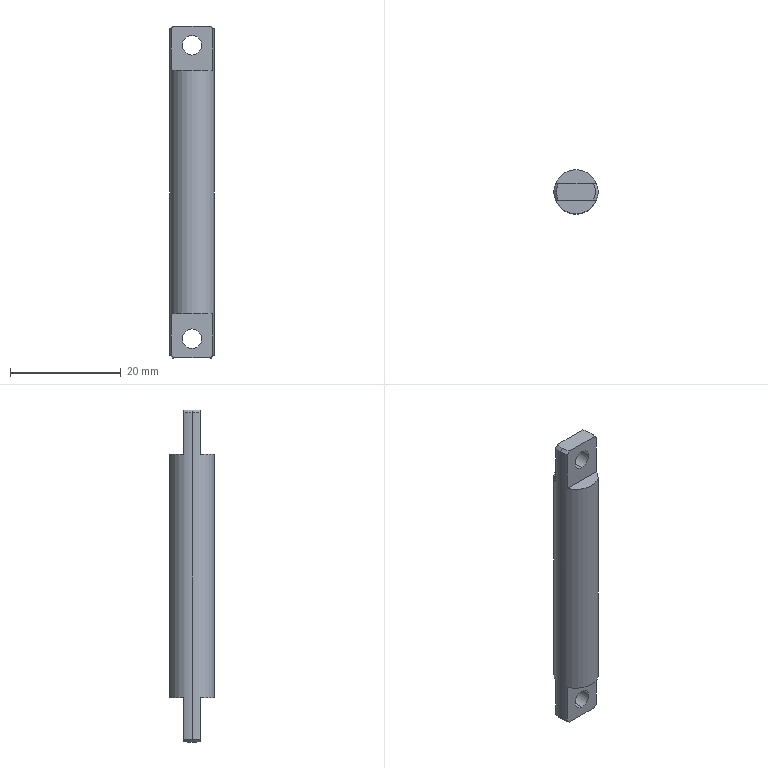Part | SolidWorks | features BaseBody 1 | 1 solid | 21 faces | box 8 x 8 x 60 mm | volume 2527 mm3 | plane 10 | cylinder 6 | cone 5 | commonest cylinder face diameters 3.5 x4 8 x2
STEP:
#1=CARTESIAN_POINT('',(4.,0.,29.5));
#2=VERTEX_POINT('',#1);
#3=CARTESIAN_POINT('',(3.708,1.5,29.5));
#4=VERTEX_POINT('',#3);
#5=CARTESIAN_POINT('',(0.,0.,29.5));
#6=DIRECTION('',(0.,0.,1.));
#7=DIRECTION('',(-1.,0.,0.));
#8=AXIS2_PLACEMENT_3D('',#5,#6,#7);
#9=CIRCLE('',#8,4.);
#10=EDGE_CURVE('',#2,#4,#9,.T.);
#11=ORIENTED_EDGE('',*,*,#10,.F.);
#12=CARTESIAN_POINT('',(4.,0.,-29.5));
#13=VERTEX_POINT('',#12);
#14=CARTESIAN_POINT('',(4.,0.,22.));
#15=DIRECTION('',(0.,0.,-1.));
#16=VECTOR('',#15,1000.);
#17=LINE('',#14,#16);
#18=EDGE_CURVE('',#2,#13,#17,.T.);
#19=ORIENTED_EDGE('',*,*,#18,.T.);
#20=CARTESIAN_POINT('',(3.708,1.5,-29.5));
#21=VERTEX_POINT('',#20);
#22=CARTESIAN_POINT('',(0.,0.,-29.5));
#23=DIRECTION('',(0.,0.,1.));
#24=DIRECTION('',(-1.,0.,0.));
#25=AXIS2_PLACEMENT_3D('',#22,#23,#24);
#26=CIRCLE('',#25,4.);
#27=EDGE_CURVE('',#13,#21,#26,.T.);
#28=ORIENTED_EDGE('',*,*,#27,.T.);
#29=CARTESIAN_POINT('',(3.708,1.5,-22.));
#30=VERTEX_POINT('',#29);
#31=CARTESIAN_POINT('',(3.708,1.5,22.));
#32=DIRECTION('',(0.,0.,1.));
#33=VECTOR('',#32,1000.);
#34=LINE('',#31,#33);
#35=EDGE_CURVE('',#21,#30,#34,.T.);
#36=ORIENTED_EDGE('',*,*,#35,.T.);
#37=CARTESIAN_POINT('',(-3.708,1.5,-22.));
#38=VERTEX_POINT('',#37);
#39=CARTESIAN_POINT('',(0.,0.,-22.));
#40=DIRECTION('',(0.,0.,1.));
#41=DIRECTION('',(-1.,0.,0.));
#42=AXIS2_PLACEMENT_3D('',#39,#40,#41);
#43=CIRCLE('',#42,4.);
#44=EDGE_CURVE('',#30,#38,#43,.T.);
#45=ORIENTED_EDGE('',*,*,#44,.T.);
#46=CARTESIAN_POINT('',(-3.708,1.5,-29.5));
#47=VERTEX_POINT('',#46);
#48=CARTESIAN_POINT('',(-3.708,1.5,22.));
#49=DIRECTION('',(0.,0.,-1.));
#50=VECTOR('',#49,1000.);
#51=LINE('',#48,#50);
#52=EDGE_CURVE('',#38,#47,#51,.T.);
#53=ORIENTED_EDGE('',*,*,#52,.T.);
#54=CARTESIAN_POINT('',(-4.,0.,-29.5));
#55=VERTEX_POINT('',#54);
#56=CARTESIAN_POINT('',(0.,0.,-29.5));
#57=DIRECTION('',(0.,0.,-1.));
#58=DIRECTION('',(1.,0.,0.));
#59=AXIS2_PLACEMENT_3D('',#56,#57,#58);
#60=CIRCLE('',#59,4.);
#61=EDGE_CURVE('',#55,#47,#60,.T.);
#62=ORIENTED_EDGE('',*,*,#61,.F.);
#63=CARTESIAN_POINT('',(-4.,0.,29.5));
#64=VERTEX_POINT('',#63);
#65=CARTESIAN_POINT('',(-4.,0.,22.));
#66=DIRECTION('',(0.,0.,-1.));
#67=VECTOR('',#66,1000.);
#68=LINE('',#65,#67);
#69=EDGE_CURVE('',#64,#55,#68,.T.);
#70=ORIENTED_EDGE('',*,*,#69,.F.);
#71=CARTESIAN_POINT('',(-3.708,1.5,29.5));
#72=VERTEX_POINT('',#71);
#73=CARTESIAN_POINT('',(0.,0.,29.5));
#74=DIRECTION('',(0.,0.,-1.));
#75=DIRECTION('',(-1.,0.,0.));
#76=AXIS2_PLACEMENT_3D('',#73,#74,#75);
#77=CIRCLE('',#76,4.);
#78=EDGE_CURVE('',#64,#72,#77,.T.);
#79=ORIENTED_EDGE('',*,*,#78,.T.);
#80=CARTESIAN_POINT('',(-3.708,1.5,22.));
#81=VERTEX_POINT('',#80);
#82=CARTESIAN_POINT('',(-3.708,1.5,22.));
#83=DIRECTION('',(0.,0.,-1.));
#84=VECTOR('',#83,1000.);
#85=LINE('',#82,#84);
#86=EDGE_CURVE('',#72,#81,#85,.T.);
#87=ORIENTED_EDGE('',*,*,#86,.T.);
#88=CARTESIAN_POINT('',(3.708,1.5,22.));
#89=VERTEX_POINT('',#88);
#90=CARTESIAN_POINT('',(0.,0.,22.));
#91=DIRECTION('',(0.,0.,-1.));
#92=DIRECTION('',(-1.,0.,0.));
#93=AXIS2_PLACEMENT_3D('',#90,#91,#92);
#94=CIRCLE('',#93,4.);
#95=EDGE_CURVE('',#81,#89,#94,.T.);
#96=ORIENTED_EDGE('',*,*,#95,.T.);
#97=CARTESIAN_POINT('',(3.708,1.5,22.));
#98=DIRECTION('',(0.,0.,1.));
#99=VECTOR('',#98,1000.);
#100=LINE('',#97,#99);
#101=EDGE_CURVE('',#89,#4,#100,.T.);
#102=ORIENTED_EDGE('',*,*,#101,.T.);
#103=EDGE_LOOP('',(#11,#19,#28,#36,#45,#53,#62,#70,#79,#87,#96,#102));
#104=FACE_OUTER_BOUND('',#103,.T.);
#105=CARTESIAN_POINT('',(0.,0.,22.));
#106=DIRECTION('',(0.,0.,-1.));
#107=DIRECTION('',(-1.,0.,0.));
#108=AXIS2_PLACEMENT_3D('',#105,#106,#107);
#109=CYLINDRICAL_SURFACE('',#108,4.);
#110=ADVANCED_FACE('',(#104),#109,.T.);
#111=CARTESIAN_POINT('',(-3.162,-1.5,30.));
#112=VERTEX_POINT('',#111);
#113=CARTESIAN_POINT('',(-3.5,0.,30.));
#114=VERTEX_POINT('',#113);
#115=CARTESIAN_POINT('',(0.,0.,30.));
#116=DIRECTION('',(0.,0.,-1.));
#117=DIRECTION('',(-1.,0.,0.));
#118=AXIS2_PLACEMENT_3D('',#115,#116,#117);
#119=CIRCLE('',#118,3.5);
#120=EDGE_CURVE('',#112,#114,#119,.T.);
#121=ORIENTED_EDGE('',*,*,#120,.T.);
#122=CARTESIAN_POINT('',(-4.,0.,29.5));
#123=DIRECTION('',(-0.7071,0.,-0.7071));
#124=VECTOR('',#123,1000.);
#125=LINE('',#122,#124);
#126=EDGE_CURVE('',#114,#64,#125,.T.);
#127=ORIENTED_EDGE('',*,*,#126,.T.);
#128=CARTESIAN_POINT('',(-3.708,-1.5,29.5));
#129=VERTEX_POINT('',#128);
#130=CARTESIAN_POINT('',(0.,0.,29.5));
#131=DIRECTION('',(0.,0.,-1.));
#132=DIRECTION('',(-1.,0.,0.));
#133=AXIS2_PLACEMENT_3D('',#130,#131,#132);
#134=CIRCLE('',#133,4.);
#135=EDGE_CURVE('',#129,#64,#134,.T.);
#136=ORIENTED_EDGE('',*,*,#135,.F.);
#137=CARTESIAN_POINT('',(-3.708,-1.5,29.5));
#138=CARTESIAN_POINT('',(-3.527,-1.5,29.668));
#139=CARTESIAN_POINT('',(-3.345,-1.5,29.835));
#140=CARTESIAN_POINT('',(-3.162,-1.5,30.));
#141=B_SPLINE_CURVE_WITH_KNOTS('',3,(#137,#138,#139,#140),.UNSPECIFIED.,.F.,.F.,(4,4),(0.,0.0007402),.UNSPECIFIED.);
#142=EDGE_CURVE('',#129,#112,#141,.T.);
#143=ORIENTED_EDGE('',*,*,#142,.T.);
#144=EDGE_LOOP('',(#121,#127,#136,#143));
#145=FACE_OUTER_BOUND('',#144,.T.);
#146=CARTESIAN_POINT('',(0.,0.,29.5));
#147=DIRECTION('',(0.,0.,-1.));
#148=DIRECTION('',(-1.,0.,0.));
#149=AXIS2_PLACEMENT_3D('',#146,#147,#148);
#150=CONICAL_SURFACE('',#149,4.,0.7854);
#151=ADVANCED_FACE('',(#145),#150,.T.);
#152=CARTESIAN_POINT('',(-0.001901,-1.5,24.75));
#153=VERTEX_POINT('',#152);
#154=CARTESIAN_POINT('',(-0.001901,-1.5,28.25));
#155=VERTEX_POINT('',#154);
#156=CARTESIAN_POINT('',(-0.001901,-1.5,26.5));
#157=DIRECTION('',(0.,1.,0.));
#158=DIRECTION('',(0.,0.,1.));
#159=AXIS2_PLACEMENT_3D('',#156,#157,#158);
#160=CIRCLE('',#159,1.75);
#161=EDGE_CURVE('',#153,#155,#160,.T.);
#162=ORIENTED_EDGE('',*,*,#161,.F.);
#163=CARTESIAN_POINT('',(-0.001901,1.5,24.75));
#164=VERTEX_POINT('',#163);
#165=CARTESIAN_POINT('',(-0.001901,1.5,24.75));
#166=DIRECTION('',(0.,1.,0.));
#167=VECTOR('',#166,1000.);
#168=LINE('',#165,#167);
#169=EDGE_CURVE('',#153,#164,#168,.T.);
#170=ORIENTED_EDGE('',*,*,#169,.T.);
#171=CARTESIAN_POINT('',(-0.001901,1.5,28.25));
#172=VERTEX_POINT('',#171);
#173=CARTESIAN_POINT('',(-0.001901,1.5,26.5));
#174=DIRECTION('',(0.,1.,0.));
#175=DIRECTION('',(0.,0.,1.));
#176=AXIS2_PLACEMENT_3D('',#173,#174,#175);
#177=CIRCLE('',#176,1.75);
#178=EDGE_CURVE('',#164,#172,#177,.T.);
#179=ORIENTED_EDGE('',*,*,#178,.T.);
#180=CARTESIAN_POINT('',(-0.001901,1.5,28.25));
#181=DIRECTION('',(0.,1.,0.));
#182=VECTOR('',#181,1000.);
#183=LINE('',#180,#182);
#184=EDGE_CURVE('',#155,#172,#183,.T.);
#185=ORIENTED_EDGE('',*,*,#184,.F.);
#186=EDGE_LOOP('',(#162,#170,#179,#185));
#187=FACE_OUTER_BOUND('',#186,.T.);
#188=CARTESIAN_POINT('',(-0.001901,1.5,26.5));
#189=DIRECTION('',(0.,1.,0.));
#190=DIRECTION('',(0.,0.,1.));
#191=AXIS2_PLACEMENT_3D('',#188,#189,#190);
#192=CYLINDRICAL_SURFACE('',#191,1.75);
#193=ADVANCED_FACE('',(#187),#192,.F.);
#194=CARTESIAN_POINT('',(-0.001901,-1.5,-28.25));
#195=VERTEX_POINT('',#194);
#196=CARTESIAN_POINT('',(-0.001901,-1.5,-24.75));
#197=VERTEX_POINT('',#196);
#198=CARTESIAN_POINT('',(-0.001901,-1.5,-26.5));
#199=DIRECTION('',(0.,1.,0.));
#200=DIRECTION('',(0.,0.,1.));
#201=AXIS2_PLACEMENT_3D('',#198,#199,#200);
#202=CIRCLE('',#201,1.75);
#203=EDGE_CURVE('',#195,#197,#202,.T.);
#204=ORIENTED_EDGE('',*,*,#203,.F.);
#205=CARTESIAN_POINT('',(-0.001901,1.5,-28.25));
#206=VERTEX_POINT('',#205);
#207=CARTESIAN_POINT('',(-0.001901,1.5,-28.25));
#208=DIRECTION('',(0.,1.,0.));
#209=VECTOR('',#208,1000.);
#210=LINE('',#207,#209);
#211=EDGE_CURVE('',#195,#206,#210,.T.);
#212=ORIENTED_EDGE('',*,*,#211,.T.);
#213=CARTESIAN_POINT('',(-0.001901,1.5,-24.75));
#214=VERTEX_POINT('',#213);
#215=CARTESIAN_POINT('',(-0.001901,1.5,-26.5));
#216=DIRECTION('',(0.,-1.,0.));
#217=DIRECTION('',(0.,0.,1.));
#218=AXIS2_PLACEMENT_3D('',#215,#216,#217);
#219=CIRCLE('',#218,1.75);
#220=EDGE_CURVE('',#214,#206,#219,.T.);
#221=ORIENTED_EDGE('',*,*,#220,.F.);
#222=CARTESIAN_POINT('',(-0.001901,1.5,-24.75));
#223=DIRECTION('',(0.,1.,0.));
#224=VECTOR('',#223,1000.);
#225=LINE('',#222,#224);
#226=EDGE_CURVE('',#197,#214,#225,.T.);
#227=ORIENTED_EDGE('',*,*,#226,.F.);
#228=EDGE_LOOP('',(#204,#212,#221,#227));
#229=FACE_OUTER_BOUND('',#228,.T.);
#230=CARTESIAN_POINT('',(-0.001901,1.5,-26.5));
#231=DIRECTION('',(0.,1.,0.));
#232=DIRECTION('',(0.,0.,1.));
#233=AXIS2_PLACEMENT_3D('',#230,#231,#232);
#234=CYLINDRICAL_SURFACE('',#233,1.75);
#235=ADVANCED_FACE('',(#229),#234,.F.);
#236=ORIENTED_EDGE('',*,*,#18,.F.);
#237=CARTESIAN_POINT('',(3.708,-1.5,29.5));
#238=VERTEX_POINT('',#237);
#239=CARTESIAN_POINT('',(0.,0.,29.5));
#240=DIRECTION('',(0.,0.,1.));
#241=DIRECTION('',(-1.,0.,0.));
#242=AXIS2_PLACEMENT_3D('',#239,#240,#241);
#243=CIRCLE('',#242,4.);
#244=EDGE_CURVE('',#238,#2,#243,.T.);
#245=ORIENTED_EDGE('',*,*,#244,.F.);
#246=CARTESIAN_POINT('',(3.708,-1.5,22.));
#247=VERTEX_POINT('',#246);
#248=CARTESIAN_POINT('',(3.708,-1.5,22.));
#249=DIRECTION('',(0.,0.,-1.));
#250=VECTOR('',#249,1000.);
#251=LINE('',#248,#250);
#252=EDGE_CURVE('',#238,#247,#251,.T.);
#253=ORIENTED_EDGE('',*,*,#252,.T.);
#254=CARTESIAN_POINT('',(-3.708,-1.5,22.));
#255=VERTEX_POINT('',#254);
#256=CARTESIAN_POINT('',(0.,0.,22.));
#257=DIRECTION('',(0.,0.,-1.));
#258=DIRECTION('',(-1.,0.,0.));
#259=AXIS2_PLACEMENT_3D('',#256,#257,#258);
#260=CIRCLE('',#259,4.);
#261=EDGE_CURVE('',#247,#255,#260,.T.);
#262=ORIENTED_EDGE('',*,*,#261,.T.);
#263=CARTESIAN_POINT('',(-3.708,-1.5,22.));
#264=DIRECTION('',(0.,0.,1.));
#265=VECTOR('',#264,1000.);
#266=LINE('',#263,#265);
#267=EDGE_CURVE('',#255,#129,#266,.T.);
#268=ORIENTED_EDGE('',*,*,#267,.T.);
#269=ORIENTED_EDGE('',*,*,#135,.T.);
#270=ORIENTED_EDGE('',*,*,#69,.T.);
#271=CARTESIAN_POINT('',(-3.708,-1.5,-29.5));
#272=VERTEX_POINT('',#271);
#273=CARTESIAN_POINT('',(0.,0.,-29.5));
#274=DIRECTION('',(0.,0.,-1.));
#275=DIRECTION('',(1.,0.,0.));
#276=AXIS2_PLACEMENT_3D('',#273,#274,#275);
#277=CIRCLE('',#276,4.);
#278=EDGE_CURVE('',#272,#55,#277,.T.);
#279=ORIENTED_EDGE('',*,*,#278,.F.);
#280=CARTESIAN_POINT('',(-3.708,-1.5,-22.));
#281=VERTEX_POINT('',#280);
#282=CARTESIAN_POINT('',(-3.708,-1.5,22.));
#283=DIRECTION('',(0.,0.,1.));
#284=VECTOR('',#283,1000.);
#285=LINE('',#282,#284);
#286=EDGE_CURVE('',#272,#281,#285,.T.);
#287=ORIENTED_EDGE('',*,*,#286,.T.);
#288=CARTESIAN_POINT('',(3.708,-1.5,-22.));
#289=VERTEX_POINT('',#288);
#290=CARTESIAN_POINT('',(0.,0.,-22.));
#291=DIRECTION('',(0.,0.,1.));
#292=DIRECTION('',(-1.,0.,0.));
#293=AXIS2_PLACEMENT_3D('',#290,#291,#292);
#294=CIRCLE('',#293,4.);
#295=EDGE_CURVE('',#281,#289,#294,.T.);
#296=ORIENTED_EDGE('',*,*,#295,.T.);
#297=CARTESIAN_POINT('',(3.708,-1.5,-29.5));
#298=VERTEX_POINT('',#297);
#299=CARTESIAN_POINT('',(3.708,-1.5,22.));
#300=DIRECTION('',(0.,0.,-1.));
#301=VECTOR('',#300,1000.);
#302=LINE('',#299,#301);
#303=EDGE_CURVE('',#289,#298,#302,.T.);
#304=ORIENTED_EDGE('',*,*,#303,.T.);
#305=CARTESIAN_POINT('',(0.,0.,-29.5));
#306=DIRECTION('',(0.,0.,1.));
#307=DIRECTION('',(-1.,0.,0.));
#308=AXIS2_PLACEMENT_3D('',#305,#306,#307);
#309=CIRCLE('',#308,4.);
#310=EDGE_CURVE('',#298,#13,#309,.T.);
#311=ORIENTED_EDGE('',*,*,#310,.T.);
#312=EDGE_LOOP('',(#236,#245,#253,#262,#268,#269,#270,#279,#287,#296,#304,#311));
#313=FACE_OUTER_BOUND('',#312,.T.);
#314=CARTESIAN_POINT('',(0.,0.,22.));
#315=DIRECTION('',(0.,0.,-1.));
#316=DIRECTION('',(-1.,0.,0.));
#317=AXIS2_PLACEMENT_3D('',#314,#315,#316);
#318=CYLINDRICAL_SURFACE('',#317,4.);
#319=ADVANCED_FACE('',(#313),#318,.T.);
#320=CARTESIAN_POINT('',(3.162,1.5,30.));
#321=VERTEX_POINT('',#320);
#322=CARTESIAN_POINT('',(3.708,1.5,29.5));
#323=CARTESIAN_POINT('',(3.527,1.5,29.668));
#324=CARTESIAN_POINT('',(3.345,1.5,29.835));
#325=CARTESIAN_POINT('',(3.162,1.5,30.));
#326=B_SPLINE_CURVE_WITH_KNOTS('',3,(#322,#323,#324,#325),.UNSPECIFIED.,.F.,.F.,(4,4),(0.,0.0007402),.UNSPECIFIED.);
#327=EDGE_CURVE('',#4,#321,#326,.T.);
#328=ORIENTED_EDGE('',*,*,#327,.F.);
#329=ORIENTED_EDGE('',*,*,#101,.F.);
#330=CARTESIAN_POINT('',(-3.708,1.5,22.));
#331=DIRECTION('',(1.,0.,0.));
#332=VECTOR('',#331,1000.);
#333=LINE('',#330,#332);
#334=EDGE_CURVE('',#81,#89,#333,.T.);
#335=ORIENTED_EDGE('',*,*,#334,.F.);
#336=ORIENTED_EDGE('',*,*,#86,.F.);
#337=CARTESIAN_POINT('',(-3.162,1.5,30.));
#338=VERTEX_POINT('',#337);
#339=CARTESIAN_POINT('',(-3.162,1.5,30.));
#340=CARTESIAN_POINT('',(-3.345,1.5,29.835));
#341=CARTESIAN_POINT('',(-3.527,1.5,29.668));
#342=CARTESIAN_POINT('',(-3.708,1.5,29.5));
#343=B_SPLINE_CURVE_WITH_KNOTS('',3,(#339,#340,#341,#342),.UNSPECIFIED.,.F.,.F.,(4,4),(0.,0.0007402),.UNSPECIFIED.);
#344=EDGE_CURVE('',#338,#72,#343,.T.);
#345=ORIENTED_EDGE('',*,*,#344,.F.);
#346=CARTESIAN_POINT('',(-3.708,1.5,30.));
#347=DIRECTION('',(-1.,0.,0.));
#348=VECTOR('',#347,1000.);
#349=LINE('',#346,#348);
#350=EDGE_CURVE('',#321,#338,#349,.T.);
#351=ORIENTED_EDGE('',*,*,#350,.F.);
#352=EDGE_LOOP('',(#328,#329,#335,#336,#345,#351));
#353=FACE_OUTER_BOUND('',#352,.T.);
#354=CARTESIAN_POINT('',(-0.001901,1.5,26.5));
#355=DIRECTION('',(0.,1.,0.));
#356=DIRECTION('',(0.,0.,1.));
#357=AXIS2_PLACEMENT_3D('',#354,#355,#356);
#358=CIRCLE('',#357,1.75);
#359=EDGE_CURVE('',#172,#164,#358,.T.);
#360=ORIENTED_EDGE('',*,*,#359,.F.);
#361=ORIENTED_EDGE('',*,*,#178,.F.);
#362=EDGE_LOOP('',(#360,#361));
#363=FACE_BOUND('',#362,.T.);
#364=CARTESIAN_POINT('',(-3.708,1.5,30.));
#365=DIRECTION('',(0.,-1.,0.));
#366=DIRECTION('',(0.,0.,-1.));
#367=AXIS2_PLACEMENT_3D('',#364,#365,#366);
#368=PLANE('',#367);
#369=ADVANCED_FACE('',(#353,#363),#368,.F.);
#370=ORIENTED_EDGE('',*,*,#334,.T.);
#371=ORIENTED_EDGE('',*,*,#95,.F.);
#372=EDGE_LOOP('',(#370,#371));
#373=FACE_OUTER_BOUND('',#372,.T.);
#374=CARTESIAN_POINT('',(0.,0.,22.));
#375=DIRECTION('',(0.,0.,1.));
#376=DIRECTION('',(1.,0.,0.));
#377=AXIS2_PLACEMENT_3D('',#374,#375,#376);
#378=PLANE('',#377);
#379=ADVANCED_FACE('',(#373),#378,.T.);
#380=ORIENTED_EDGE('',*,*,#126,.F.);
#381=CARTESIAN_POINT('',(0.,0.,30.));
#382=DIRECTION('',(0.,0.,-1.));
#383=DIRECTION('',(-1.,0.,0.));
#384=AXIS2_PLACEMENT_3D('',#381,#382,#383);
#385=CIRCLE('',#384,3.5);
#386=EDGE_CURVE('',#114,#338,#385,.T.);
#387=ORIENTED_EDGE('',*,*,#386,.T.);
#388=ORIENTED_EDGE('',*,*,#344,.T.);
#389=ORIENTED_EDGE('',*,*,#78,.F.);
#390=EDGE_LOOP('',(#380,#387,#388,#389));
#391=FACE_OUTER_BOUND('',#390,.T.);
#392=CARTESIAN_POINT('',(0.,0.,29.5));
#393=DIRECTION('',(0.,0.,-1.));
#394=DIRECTION('',(-1.,0.,0.));
#395=AXIS2_PLACEMENT_3D('',#392,#393,#394);
#396=CONICAL_SURFACE('',#395,4.,0.7854);
#397=ADVANCED_FACE('',(#391),#396,.T.);
#398=ORIENTED_EDGE('',*,*,#52,.F.);
#399=CARTESIAN_POINT('',(-3.708,1.5,-22.));
#400=DIRECTION('',(1.,0.,0.));
#401=VECTOR('',#400,1000.);
#402=LINE('',#399,#401);
#403=EDGE_CURVE('',#38,#30,#402,.T.);
#404=ORIENTED_EDGE('',*,*,#403,.T.);
#405=ORIENTED_EDGE('',*,*,#35,.F.);
#406=CARTESIAN_POINT('',(3.162,1.5,-30.));
#407=VERTEX_POINT('',#406);
#408=CARTESIAN_POINT('',(3.708,1.5,-29.5));
#409=CARTESIAN_POINT('',(3.527,1.5,-29.668));
#410=CARTESIAN_POINT('',(3.345,1.5,-29.835));
#411=CARTESIAN_POINT('',(3.162,1.5,-30.));
#412=B_SPLINE_CURVE_WITH_KNOTS('',3,(#408,#409,#410,#411),.UNSPECIFIED.,.F.,.F.,(4,4),(0.,0.0007402),.UNSPECIFIED.);
#413=EDGE_CURVE('',#21,#407,#412,.T.);
#414=ORIENTED_EDGE('',*,*,#413,.T.);
#415=CARTESIAN_POINT('',(-3.162,1.5,-30.));
#416=VERTEX_POINT('',#415);
#417=CARTESIAN_POINT('',(-3.708,1.5,-30.));
#418=DIRECTION('',(-1.,0.,0.));
#419=VECTOR('',#418,1000.);
#420=LINE('',#417,#419);
#421=EDGE_CURVE('',#407,#416,#420,.T.);
#422=ORIENTED_EDGE('',*,*,#421,.T.);
#423=CARTESIAN_POINT('',(-3.708,1.5,-29.5));
#424=CARTESIAN_POINT('',(-3.527,1.5,-29.668));
#425=CARTESIAN_POINT('',(-3.345,1.5,-29.835));
#426=CARTESIAN_POINT('',(-3.162,1.5,-30.));
#427=B_SPLINE_CURVE_WITH_KNOTS('',3,(#423,#424,#425,#426),.UNSPECIFIED.,.F.,.F.,(4,4),(0.,0.0007402),.UNSPECIFIED.);
#428=EDGE_CURVE('',#47,#416,#427,.T.);
#429=ORIENTED_EDGE('',*,*,#428,.F.);
#430=EDGE_LOOP('',(#398,#404,#405,#414,#422,#429));
#431=FACE_OUTER_BOUND('',#430,.T.);
#432=ORIENTED_EDGE('',*,*,#220,.T.);
#433=CARTESIAN_POINT('',(-0.001901,1.5,-26.5));
#434=DIRECTION('',(0.,-1.,0.));
#435=DIRECTION('',(0.,0.,1.));
#436=AXIS2_PLACEMENT_3D('',#433,#434,#435);
#437=CIRCLE('',#436,1.75);
#438=EDGE_CURVE('',#206,#214,#437,.T.);
#439=ORIENTED_EDGE('',*,*,#438,.T.);
#440=EDGE_LOOP('',(#432,#439));
#441=FACE_BOUND('',#440,.T.);
#442=CARTESIAN_POINT('',(-3.708,1.5,-30.));
#443=DIRECTION('',(0.,1.,0.));
#444=DIRECTION('',(0.,0.,1.));
#445=AXIS2_PLACEMENT_3D('',#442,#443,#444);
#446=PLANE('',#445);
#447=ADVANCED_FACE('',(#431,#441),#446,.T.);
#448=ORIENTED_EDGE('',*,*,#403,.F.);
#449=ORIENTED_EDGE('',*,*,#44,.F.);
#450=EDGE_LOOP('',(#448,#449));
#451=FACE_OUTER_BOUND('',#450,.T.);
#452=CARTESIAN_POINT('',(0.,0.,-22.));
#453=DIRECTION('',(0.,0.,1.));
#454=DIRECTION('',(1.,0.,0.));
#455=AXIS2_PLACEMENT_3D('',#452,#453,#454);
#456=PLANE('',#455);
#457=ADVANCED_FACE('',(#451),#456,.F.);
#458=ORIENTED_EDGE('',*,*,#413,.F.);
#459=ORIENTED_EDGE('',*,*,#27,.F.);
#460=ORIENTED_EDGE('',*,*,#310,.F.);
#461=CARTESIAN_POINT('',(3.162,-1.5,-30.));
#462=VERTEX_POINT('',#461);
#463=CARTESIAN_POINT('',(3.708,-1.5,-29.5));
#464=CARTESIAN_POINT('',(3.527,-1.5,-29.668));
#465=CARTESIAN_POINT('',(3.345,-1.5,-29.835));
#466=CARTESIAN_POINT('',(3.162,-1.5,-30.));
#467=B_SPLINE_CURVE_WITH_KNOTS('',3,(#463,#464,#465,#466),.UNSPECIFIED.,.F.,.F.,(4,4),(0.,0.0007402),.UNSPECIFIED.);
#468=EDGE_CURVE('',#298,#462,#467,.T.);
#469=ORIENTED_EDGE('',*,*,#468,.T.);
#470=CARTESIAN_POINT('',(0.,0.,-30.));
#471=DIRECTION('',(0.,0.,1.));
#472=DIRECTION('',(0.,-1.,0.));
#473=AXIS2_PLACEMENT_3D('',#470,#471,#472);
#474=CIRCLE('',#473,3.5);
#475=EDGE_CURVE('',#462,#407,#474,.T.);
#476=ORIENTED_EDGE('',*,*,#475,.T.);
#477=EDGE_LOOP('',(#458,#459,#460,#469,#476));
#478=FACE_OUTER_BOUND('',#477,.T.);
#479=CARTESIAN_POINT('',(0.,0.,-29.5));
#480=DIRECTION('',(0.,0.,1.));
#481=DIRECTION('',(0.,-1.,0.));
#482=AXIS2_PLACEMENT_3D('',#479,#480,#481);
#483=CONICAL_SURFACE('',#482,4.,0.7854);
#484=ADVANCED_FACE('',(#478),#483,.T.);
#485=CARTESIAN_POINT('',(3.162,-1.5,30.));
#486=VERTEX_POINT('',#485);
#487=CARTESIAN_POINT('',(0.,0.,30.));
#488=DIRECTION('',(0.,0.,-1.));
#489=DIRECTION('',(-1.,0.,0.));
#490=AXIS2_PLACEMENT_3D('',#487,#488,#489);
#491=CIRCLE('',#490,3.5);
#492=EDGE_CURVE('',#321,#486,#491,.T.);
#493=ORIENTED_EDGE('',*,*,#492,.F.);
#494=ORIENTED_EDGE('',*,*,#350,.T.);
#495=ORIENTED_EDGE('',*,*,#386,.F.);
#496=ORIENTED_EDGE('',*,*,#120,.F.);
#497=CARTESIAN_POINT('',(0.,-1.5,30.));
#498=DIRECTION('',(-1.,0.,0.));
#499=VECTOR('',#498,1000.);
#500=LINE('',#497,#499);
#501=EDGE_CURVE('',#486,#112,#500,.T.);
#502=ORIENTED_EDGE('',*,*,#501,.F.);
#503=EDGE_LOOP('',(#493,#494,#495,#496,#502));
#504=FACE_OUTER_BOUND('',#503,.T.);
#505=CARTESIAN_POINT('',(0.,0.,30.));
#506=DIRECTION('',(0.,0.,-1.));
#507=DIRECTION('',(-1.,0.,0.));
#508=AXIS2_PLACEMENT_3D('',#505,#506,#507);
#509=PLANE('',#508);
#510=ADVANCED_FACE('',(#504),#509,.F.);
#511=ORIENTED_EDGE('',*,*,#169,.F.);
#512=CARTESIAN_POINT('',(-0.001901,-1.5,26.5));
#513=DIRECTION('',(0.,1.,0.));
#514=DIRECTION('',(0.,0.,1.));
#515=AXIS2_PLACEMENT_3D('',#512,#513,#514);
#516=CIRCLE('',#515,1.75);
#517=EDGE_CURVE('',#155,#153,#516,.T.);
#518=ORIENTED_EDGE('',*,*,#517,.F.);
#519=ORIENTED_EDGE('',*,*,#184,.T.);
#520=ORIENTED_EDGE('',*,*,#359,.T.);
#521=EDGE_LOOP('',(#511,#518,#519,#520));
#522=FACE_OUTER_BOUND('',#521,.T.);
#523=CARTESIAN_POINT('',(-0.001901,1.5,26.5));
#524=DIRECTION('',(0.,1.,0.));
#525=DIRECTION('',(0.,0.,1.));
#526=AXIS2_PLACEMENT_3D('',#523,#524,#525);
#527=CYLINDRICAL_SURFACE('',#526,1.75);
#528=ADVANCED_FACE('',(#522),#527,.F.);
#529=ORIENTED_EDGE('',*,*,#286,.F.);
#530=CARTESIAN_POINT('',(-3.162,-1.5,-30.));
#531=VERTEX_POINT('',#530);
#532=CARTESIAN_POINT('',(-3.162,-1.5,-30.));
#533=CARTESIAN_POINT('',(-3.345,-1.5,-29.835));
#534=CARTESIAN_POINT('',(-3.527,-1.5,-29.668));
#535=CARTESIAN_POINT('',(-3.708,-1.5,-29.5));
#536=B_SPLINE_CURVE_WITH_KNOTS('',3,(#532,#533,#534,#535),.UNSPECIFIED.,.F.,.F.,(4,4),(0.,0.0007402),.UNSPECIFIED.);
#537=EDGE_CURVE('',#531,#272,#536,.T.);
#538=ORIENTED_EDGE('',*,*,#537,.F.);
#539=CARTESIAN_POINT('',(-3.708,-1.5,-30.));
#540=DIRECTION('',(1.,0.,0.));
#541=VECTOR('',#540,1000.);
#542=LINE('',#539,#541);
#543=EDGE_CURVE('',#531,#462,#542,.T.);
#544=ORIENTED_EDGE('',*,*,#543,.T.);
#545=ORIENTED_EDGE('',*,*,#468,.F.);
#546=ORIENTED_EDGE('',*,*,#303,.F.);
#547=CARTESIAN_POINT('',(-3.708,-1.5,-22.));
#548=DIRECTION('',(-1.,0.,0.));
#549=VECTOR('',#548,1000.);
#550=LINE('',#547,#549);
#551=EDGE_CURVE('',#289,#281,#550,.T.);
#552=ORIENTED_EDGE('',*,*,#551,.T.);
#553=EDGE_LOOP('',(#529,#538,#544,#545,#546,#552));
#554=FACE_OUTER_BOUND('',#553,.T.);
#555=CARTESIAN_POINT('',(-0.001901,-1.5,-26.5));
#556=DIRECTION('',(0.,1.,0.));
#557=DIRECTION('',(0.,0.,1.));
#558=AXIS2_PLACEMENT_3D('',#555,#556,#557);
#559=CIRCLE('',#558,1.75);
#560=EDGE_CURVE('',#197,#195,#559,.T.);
#561=ORIENTED_EDGE('',*,*,#560,.T.);
#562=ORIENTED_EDGE('',*,*,#203,.T.);
#563=EDGE_LOOP('',(#561,#562));
#564=FACE_BOUND('',#563,.T.);
#565=CARTESIAN_POINT('',(-3.708,-1.5,-30.));
#566=DIRECTION('',(0.,-1.,0.));
#567=DIRECTION('',(0.,0.,-1.));
#568=AXIS2_PLACEMENT_3D('',#565,#566,#567);
#569=PLANE('',#568);
#570=ADVANCED_FACE('',(#554,#564),#569,.T.);
#571=ORIENTED_EDGE('',*,*,#551,.F.);
#572=ORIENTED_EDGE('',*,*,#295,.F.);
#573=EDGE_LOOP('',(#571,#572));
#574=FACE_OUTER_BOUND('',#573,.T.);
#575=CARTESIAN_POINT('',(0.,0.,-22.));
#576=DIRECTION('',(0.,0.,1.));
#577=DIRECTION('',(1.,0.,0.));
#578=AXIS2_PLACEMENT_3D('',#575,#576,#577);
#579=PLANE('',#578);
#580=ADVANCED_FACE('',(#574),#579,.F.);
#581=CARTESIAN_POINT('',(3.162,-1.5,30.));
#582=CARTESIAN_POINT('',(3.345,-1.5,29.835));
#583=CARTESIAN_POINT('',(3.527,-1.5,29.668));
#584=CARTESIAN_POINT('',(3.708,-1.5,29.5));
#585=B_SPLINE_CURVE_WITH_KNOTS('',3,(#581,#582,#583,#584),.UNSPECIFIED.,.F.,.F.,(4,4),(0.,0.0007402),.UNSPECIFIED.);
#586=EDGE_CURVE('',#486,#238,#585,.T.);
#587=ORIENTED_EDGE('',*,*,#586,.F.);
#588=ORIENTED_EDGE('',*,*,#501,.T.);
#589=ORIENTED_EDGE('',*,*,#142,.F.);
#590=ORIENTED_EDGE('',*,*,#267,.F.);
#591=CARTESIAN_POINT('',(-3.708,-1.5,22.));
#592=DIRECTION('',(-1.,0.,0.));
#593=VECTOR('',#592,1000.);
#594=LINE('',#591,#593);
#595=EDGE_CURVE('',#247,#255,#594,.T.);
#596=ORIENTED_EDGE('',*,*,#595,.F.);
#597=ORIENTED_EDGE('',*,*,#252,.F.);
#598=EDGE_LOOP('',(#587,#588,#589,#590,#596,#597));
#599=FACE_OUTER_BOUND('',#598,.T.);
#600=ORIENTED_EDGE('',*,*,#517,.T.);
#601=ORIENTED_EDGE('',*,*,#161,.T.);
#602=EDGE_LOOP('',(#600,#601));
#603=FACE_BOUND('',#602,.T.);
#604=CARTESIAN_POINT('',(-3.708,-1.5,30.));
#605=DIRECTION('',(0.,1.,0.));
#606=DIRECTION('',(0.,0.,1.));
#607=AXIS2_PLACEMENT_3D('',#604,#605,#606);
#608=PLANE('',#607);
#609=ADVANCED_FACE('',(#599,#603),#608,.F.);
#610=ORIENTED_EDGE('',*,*,#595,.T.);
#611=ORIENTED_EDGE('',*,*,#261,.F.);
#612=EDGE_LOOP('',(#610,#611));
#613=FACE_OUTER_BOUND('',#612,.T.);
#614=CARTESIAN_POINT('',(0.,0.,22.));
#615=DIRECTION('',(0.,0.,1.));
#616=DIRECTION('',(1.,0.,0.));
#617=AXIS2_PLACEMENT_3D('',#614,#615,#616);
#618=PLANE('',#617);
#619=ADVANCED_FACE('',(#613),#618,.T.);
#620=ORIENTED_EDGE('',*,*,#475,.F.);
#621=ORIENTED_EDGE('',*,*,#543,.F.);
#622=CARTESIAN_POINT('',(0.,0.,-30.));
#623=DIRECTION('',(0.,0.,1.));
#624=DIRECTION('',(0.,-1.,0.));
#625=AXIS2_PLACEMENT_3D('',#622,#623,#624);
#626=CIRCLE('',#625,3.5);
#627=EDGE_CURVE('',#416,#531,#626,.T.);
#628=ORIENTED_EDGE('',*,*,#627,.F.);
#629=ORIENTED_EDGE('',*,*,#421,.F.);
#630=EDGE_LOOP('',(#620,#621,#628,#629));
#631=FACE_OUTER_BOUND('',#630,.T.);
#632=CARTESIAN_POINT('',(0.,0.,-30.));
#633=DIRECTION('',(0.,0.,1.));
#634=DIRECTION('',(1.,0.,0.));
#635=AXIS2_PLACEMENT_3D('',#632,#633,#634);
#636=PLANE('',#635);
#637=ADVANCED_FACE('',(#631),#636,.F.);
#638=ORIENTED_EDGE('',*,*,#211,.F.);
#639=ORIENTED_EDGE('',*,*,#560,.F.);
#640=ORIENTED_EDGE('',*,*,#226,.T.);
#641=ORIENTED_EDGE('',*,*,#438,.F.);
#642=EDGE_LOOP('',(#638,#639,#640,#641));
#643=FACE_OUTER_BOUND('',#642,.T.);
#644=CARTESIAN_POINT('',(-0.001901,1.5,-26.5));
#645=DIRECTION('',(0.,1.,0.));
#646=DIRECTION('',(0.,0.,1.));
#647=AXIS2_PLACEMENT_3D('',#644,#645,#646);
#648=CYLINDRICAL_SURFACE('',#647,1.75);
#649=ADVANCED_FACE('',(#643),#648,.F.);
#650=ORIENTED_EDGE('',*,*,#327,.T.);
#651=ORIENTED_EDGE('',*,*,#492,.T.);
#652=ORIENTED_EDGE('',*,*,#586,.T.);
#653=ORIENTED_EDGE('',*,*,#244,.T.);
#654=ORIENTED_EDGE('',*,*,#10,.T.);
#655=EDGE_LOOP('',(#650,#651,#652,#653,#654));
#656=FACE_OUTER_BOUND('',#655,.T.);
#657=CARTESIAN_POINT('',(0.,0.,29.5));
#658=DIRECTION('',(0.,0.,-1.));
#659=DIRECTION('',(-1.,0.,0.));
#660=AXIS2_PLACEMENT_3D('',#657,#658,#659);
#661=CONICAL_SURFACE('',#660,4.,0.7854);
#662=ADVANCED_FACE('',(#656),#661,.T.);
#663=ORIENTED_EDGE('',*,*,#537,.T.);
#664=ORIENTED_EDGE('',*,*,#278,.T.);
#665=ORIENTED_EDGE('',*,*,#61,.T.);
#666=ORIENTED_EDGE('',*,*,#428,.T.);
#667=ORIENTED_EDGE('',*,*,#627,.T.);
#668=EDGE_LOOP('',(#663,#664,#665,#666,#667));
#669=FACE_OUTER_BOUND('',#668,.T.);
#670=CARTESIAN_POINT('',(0.,0.,-29.5));
#671=DIRECTION('',(0.,0.,1.));
#672=DIRECTION('',(0.,-1.,0.));
#673=AXIS2_PLACEMENT_3D('',#670,#671,#672);
#674=CONICAL_SURFACE('',#673,4.,0.7854);
#675=ADVANCED_FACE('',(#669),#674,.T.);
#676=CLOSED_SHELL('',(#110,#151,#193,#235,#319,#369,#379,#397,#447,#457,#484,#510,#528,#570,#580,#609,#619,#637,#649,#662,#675));
#677=MANIFOLD_SOLID_BREP('',#676);
#678=CARTESIAN_POINT('',(0.,0.,0.));
#679=DIRECTION('',(0.,0.,1.));
#680=DIRECTION('',(1.,0.,0.));
#681=AXIS2_PLACEMENT_3D('',#678,#679,#680);
#682=(LENGTH_UNIT()NAMED_UNIT(*)SI_UNIT(.MILLI.,.METRE.));
#683=UNCERTAINTY_MEASURE_WITH_UNIT(LENGTH_MEASURE(0.00001),#682,'','');
#684=(NAMED_UNIT(*)PLANE_ANGLE_UNIT()SI_UNIT($,.RADIAN.));
#685=(NAMED_UNIT(*)SI_UNIT($,.STERADIAN.)SOLID_ANGLE_UNIT());
#686=(GEOMETRIC_REPRESENTATION_CONTEXT(3)GLOBAL_UNCERTAINTY_ASSIGNED_CONTEXT((#683))GLOBAL_UNIT_ASSIGNED_CONTEXT((#682,#684,#685))REPRESENTATION_CONTEXT('',''));
#687=ADVANCED_BREP_SHAPE_REPRESENTATION('',(#677,#681),#686);